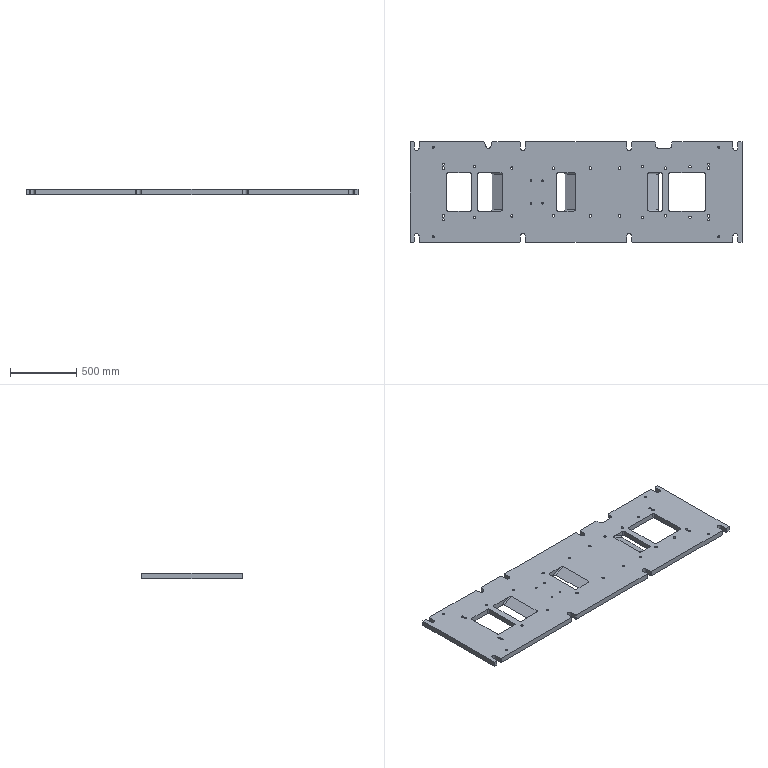Part | NX | features B1-1 2 | 1 solid | 196 faces | box 2500 x 760 x 40 mm | volume 65385915 mm3 | plane 105 | cylinder 91 | commonest cylinder face diameters 20 x24 18 x20 26 x20 16 x8 36 x8 13.5 x4